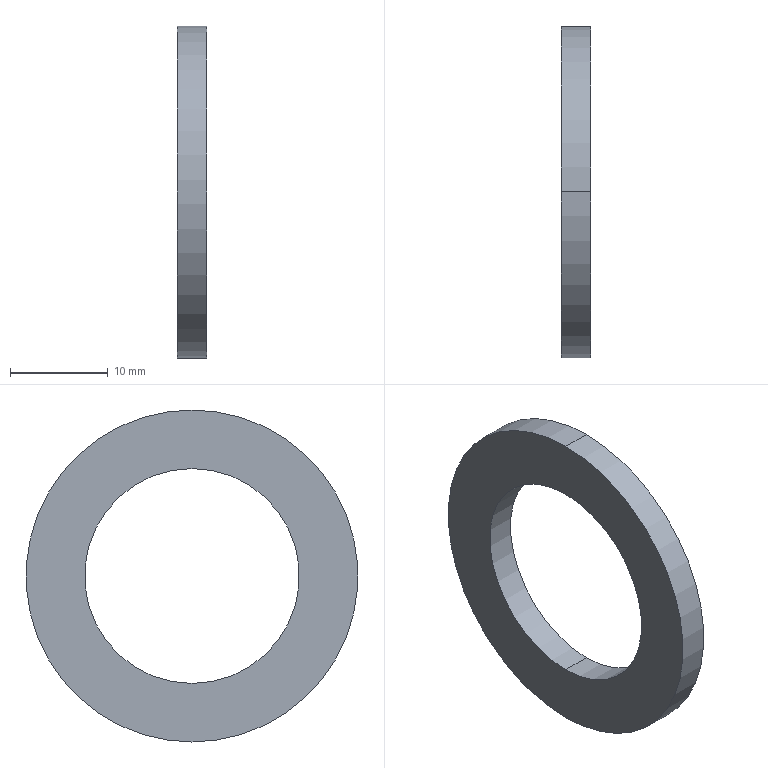Part | STEP file | Completa.sldasm-Part-113_Valor predeterminado | 1 solid | 6 faces | box 3 x 34 x 34 mm | volume 1583 mm3 | cylinder 4 | plane 2 | commonest cylinder face diameters 22 x2 34 x2
STEP:
#1=CARTESIAN_POINT('',(0.,0.,0.));
#2=DIRECTION('',(0.,0.,1.));
#3=DIRECTION('',(1.,0.,0.));
#4=AXIS2_PLACEMENT_3D('',#1,#2,#3);
#5=CARTESIAN_POINT('',(-203.167,0.,17.));
#6=VERTEX_POINT('',#5);
#7=CARTESIAN_POINT('',(-203.167,0.,-17.));
#8=VERTEX_POINT('',#7);
#9=CARTESIAN_POINT('',(-203.167,0.,0.));
#10=DIRECTION('',(-1.,0.,0.));
#11=DIRECTION('',(0.,0.,1.));
#12=AXIS2_PLACEMENT_3D('',#9,#10,#11);
#13=CIRCLE('',#12,17.);
#14=CARTESIAN_POINT('',(-203.167,0.,0.));
#15=DIRECTION('',(-1.,0.,0.));
#16=DIRECTION('',(0.,0.,1.));
#17=AXIS2_PLACEMENT_3D('',#14,#15,#16);
#18=CYLINDRICAL_SURFACE('',#17,17.);
#19=CARTESIAN_POINT('',(0.,0.));
#20=DIRECTION('',(1.,0.));
#21=VECTOR('',#20,1.);
#22=LINE('',#19,#21);
#23=(GEOMETRIC_REPRESENTATION_CONTEXT(2)PARAMETRIC_REPRESENTATION_CONTEXT()REPRESENTATION_CONTEXT('',''));
#24=DEFINITIONAL_REPRESENTATION('',(#22),#23);
#25=PCURVE('',#18,#24);
#26=CARTESIAN_POINT('',(-203.167,0.,0.));
#27=DIRECTION('',(1.,0.,0.));
#28=DIRECTION('',(0.,0.,-1.));
#29=AXIS2_PLACEMENT_3D('',#26,#27,#28);
#30=PLANE('',#29);
#31=CARTESIAN_POINT('',(-17.,0.));
#32=CARTESIAN_POINT('',(-17.,29.445));
#33=CARTESIAN_POINT('',(8.5,14.722));
#34=CARTESIAN_POINT('',(34.,0.));
#35=CARTESIAN_POINT('',(8.5,-14.722));
#36=CARTESIAN_POINT('',(-17.,-29.445));
#37=CARTESIAN_POINT('',(-17.,0.));
#38=(BOUNDED_CURVE()B_SPLINE_CURVE(2,(#31,#32,#33,#34,#35,#36,#37),.UNSPECIFIED.,.T.,.F.)B_SPLINE_CURVE_WITH_KNOTS((1,2,2,2,2,1),(-2.094,0.,2.094,4.189,6.283,8.378),.UNSPECIFIED.)CURVE()GEOMETRIC_REPRESENTATION_ITEM()RATIONAL_B_SPLINE_CURVE((1.,0.5,1.,0.5,1.,0.5,1.))REPRESENTATION_ITEM(''));
#39=(GEOMETRIC_REPRESENTATION_CONTEXT(2)PARAMETRIC_REPRESENTATION_CONTEXT()REPRESENTATION_CONTEXT('',''));
#40=DEFINITIONAL_REPRESENTATION('',(#38),#39);
#41=PCURVE('',#30,#40);
#42=SURFACE_CURVE('',#13,(#25,#41),.PCURVE_S1.);
#43=EDGE_CURVE('',#6,#8,#42,.T.);
#44=ORIENTED_EDGE('',*,*,#43,.T.);
#45=CARTESIAN_POINT('',(-206.167,0.,-17.));
#46=VERTEX_POINT('',#45);
#47=CARTESIAN_POINT('',(-203.167,0.,-17.));
#48=DIRECTION('',(-1.,0.,0.));
#49=VECTOR('',#48,1.);
#50=LINE('',#47,#49);
#51=CARTESIAN_POINT('',(3.142,0.));
#52=DIRECTION('',(0.,1.));
#53=VECTOR('',#52,1.);
#54=LINE('',#51,#53);
#55=(GEOMETRIC_REPRESENTATION_CONTEXT(2)PARAMETRIC_REPRESENTATION_CONTEXT()REPRESENTATION_CONTEXT('',''));
#56=DEFINITIONAL_REPRESENTATION('',(#54),#55);
#57=PCURVE('',#18,#56);
#58=CARTESIAN_POINT('',(-203.167,0.,0.));
#59=DIRECTION('',(-1.,0.,0.));
#60=DIRECTION('',(0.,0.,1.));
#61=AXIS2_PLACEMENT_3D('',#58,#59,#60);
#62=CYLINDRICAL_SURFACE('',#61,17.);
#63=CARTESIAN_POINT('',(3.142,0.));
#64=DIRECTION('',(0.,1.));
#65=VECTOR('',#64,1.);
#66=LINE('',#63,#65);
#67=(GEOMETRIC_REPRESENTATION_CONTEXT(2)PARAMETRIC_REPRESENTATION_CONTEXT()REPRESENTATION_CONTEXT('',''));
#68=DEFINITIONAL_REPRESENTATION('',(#66),#67);
#69=PCURVE('',#62,#68);
#70=SURFACE_CURVE('',#50,(#57,#69),.PCURVE_S1.);
#71=EDGE_CURVE('',#8,#46,#70,.T.);
#72=ORIENTED_EDGE('',*,*,#71,.T.);
#73=CARTESIAN_POINT('',(-206.167,0.,17.));
#74=VERTEX_POINT('',#73);
#75=CARTESIAN_POINT('',(-206.167,0.,0.));
#76=DIRECTION('',(-1.,0.,0.));
#77=DIRECTION('',(0.,0.,1.));
#78=AXIS2_PLACEMENT_3D('',#75,#76,#77);
#79=CIRCLE('',#78,17.);
#80=CARTESIAN_POINT('',(0.,3.));
#81=DIRECTION('',(1.,0.));
#82=VECTOR('',#81,1.);
#83=LINE('',#80,#82);
#84=(GEOMETRIC_REPRESENTATION_CONTEXT(2)PARAMETRIC_REPRESENTATION_CONTEXT()REPRESENTATION_CONTEXT('',''));
#85=DEFINITIONAL_REPRESENTATION('',(#83),#84);
#86=PCURVE('',#18,#85);
#87=CARTESIAN_POINT('',(-206.167,0.,0.));
#88=DIRECTION('',(1.,0.,0.));
#89=DIRECTION('',(0.,0.,-1.));
#90=AXIS2_PLACEMENT_3D('',#87,#88,#89);
#91=PLANE('',#90);
#92=CARTESIAN_POINT('',(-17.,0.));
#93=CARTESIAN_POINT('',(-17.,29.445));
#94=CARTESIAN_POINT('',(8.5,14.722));
#95=CARTESIAN_POINT('',(34.,0.));
#96=CARTESIAN_POINT('',(8.5,-14.722));
#97=CARTESIAN_POINT('',(-17.,-29.445));
#98=CARTESIAN_POINT('',(-17.,0.));
#99=(BOUNDED_CURVE()B_SPLINE_CURVE(2,(#92,#93,#94,#95,#96,#97,#98),.UNSPECIFIED.,.T.,.F.)B_SPLINE_CURVE_WITH_KNOTS((1,2,2,2,2,1),(-2.094,0.,2.094,4.189,6.283,8.378),.UNSPECIFIED.)CURVE()GEOMETRIC_REPRESENTATION_ITEM()RATIONAL_B_SPLINE_CURVE((1.,0.5,1.,0.5,1.,0.5,1.))REPRESENTATION_ITEM(''));
#100=(GEOMETRIC_REPRESENTATION_CONTEXT(2)PARAMETRIC_REPRESENTATION_CONTEXT()REPRESENTATION_CONTEXT('',''));
#101=DEFINITIONAL_REPRESENTATION('',(#99),#100);
#102=PCURVE('',#91,#101);
#103=SURFACE_CURVE('',#79,(#86,#102),.PCURVE_S1.);
#104=EDGE_CURVE('',#74,#46,#103,.T.);
#105=ORIENTED_EDGE('',*,*,#104,.F.);
#106=CARTESIAN_POINT('',(-203.167,0.,17.));
#107=DIRECTION('',(-1.,0.,0.));
#108=VECTOR('',#107,1.);
#109=LINE('',#106,#108);
#110=CARTESIAN_POINT('',(0.,0.));
#111=DIRECTION('',(0.,1.));
#112=VECTOR('',#111,1.);
#113=LINE('',#110,#112);
#114=(GEOMETRIC_REPRESENTATION_CONTEXT(2)PARAMETRIC_REPRESENTATION_CONTEXT()REPRESENTATION_CONTEXT('',''));
#115=DEFINITIONAL_REPRESENTATION('',(#113),#114);
#116=PCURVE('',#18,#115);
#117=CARTESIAN_POINT('',(6.283,0.));
#118=DIRECTION('',(0.,1.));
#119=VECTOR('',#118,1.);
#120=LINE('',#117,#119);
#121=(GEOMETRIC_REPRESENTATION_CONTEXT(2)PARAMETRIC_REPRESENTATION_CONTEXT()REPRESENTATION_CONTEXT('',''));
#122=DEFINITIONAL_REPRESENTATION('',(#120),#121);
#123=PCURVE('',#62,#122);
#124=SURFACE_CURVE('',#109,(#116,#123),.PCURVE_S1.);
#125=EDGE_CURVE('',#6,#74,#124,.T.);
#126=ORIENTED_EDGE('',*,*,#125,.F.);
#127=EDGE_LOOP('',(#44,#72,#105,#126));
#128=FACE_BOUND('',#127,.T.);
#129=ADVANCED_FACE('',(#128),#18,.T.);
#130=CARTESIAN_POINT('',(-203.167,0.,11.));
#131=VERTEX_POINT('',#130);
#132=CARTESIAN_POINT('',(-206.167,0.,11.));
#133=VERTEX_POINT('',#132);
#134=CARTESIAN_POINT('',(-203.167,0.,11.));
#135=DIRECTION('',(-1.,0.,0.));
#136=VECTOR('',#135,1.);
#137=LINE('',#134,#136);
#138=CARTESIAN_POINT('',(-203.167,0.,0.));
#139=DIRECTION('',(-1.,0.,0.));
#140=DIRECTION('',(0.,0.,1.));
#141=AXIS2_PLACEMENT_3D('',#138,#139,#140);
#142=CYLINDRICAL_SURFACE('',#141,11.);
#143=CARTESIAN_POINT('',(6.283,0.));
#144=DIRECTION('',(0.,1.));
#145=VECTOR('',#144,1.);
#146=LINE('',#143,#145);
#147=(GEOMETRIC_REPRESENTATION_CONTEXT(2)PARAMETRIC_REPRESENTATION_CONTEXT()REPRESENTATION_CONTEXT('',''));
#148=DEFINITIONAL_REPRESENTATION('',(#146),#147);
#149=PCURVE('',#142,#148);
#150=CARTESIAN_POINT('',(-203.167,0.,0.));
#151=DIRECTION('',(-1.,0.,0.));
#152=DIRECTION('',(0.,0.,1.));
#153=AXIS2_PLACEMENT_3D('',#150,#151,#152);
#154=CYLINDRICAL_SURFACE('',#153,11.);
#155=CARTESIAN_POINT('',(0.,0.));
#156=DIRECTION('',(0.,1.));
#157=VECTOR('',#156,1.);
#158=LINE('',#155,#157);
#159=(GEOMETRIC_REPRESENTATION_CONTEXT(2)PARAMETRIC_REPRESENTATION_CONTEXT()REPRESENTATION_CONTEXT('',''));
#160=DEFINITIONAL_REPRESENTATION('',(#158),#159);
#161=PCURVE('',#154,#160);
#162=SURFACE_CURVE('',#137,(#149,#161),.PCURVE_S1.);
#163=EDGE_CURVE('',#131,#133,#162,.T.);
#164=ORIENTED_EDGE('',*,*,#163,.T.);
#165=CARTESIAN_POINT('',(-206.167,0.,-11.));
#166=VERTEX_POINT('',#165);
#167=CARTESIAN_POINT('',(-206.167,0.,0.));
#168=DIRECTION('',(-1.,0.,0.));
#169=DIRECTION('',(0.,0.,1.));
#170=AXIS2_PLACEMENT_3D('',#167,#168,#169);
#171=CIRCLE('',#170,11.);
#172=CARTESIAN_POINT('',(0.,3.));
#173=DIRECTION('',(1.,0.));
#174=VECTOR('',#173,1.);
#175=LINE('',#172,#174);
#176=(GEOMETRIC_REPRESENTATION_CONTEXT(2)PARAMETRIC_REPRESENTATION_CONTEXT()REPRESENTATION_CONTEXT('',''));
#177=DEFINITIONAL_REPRESENTATION('',(#175),#176);
#178=PCURVE('',#142,#177);
#179=CARTESIAN_POINT('',(-11.,0.));
#180=CARTESIAN_POINT('',(-11.,19.053));
#181=CARTESIAN_POINT('',(5.5,9.526));
#182=CARTESIAN_POINT('',(22.,0.));
#183=CARTESIAN_POINT('',(5.5,-9.526));
#184=CARTESIAN_POINT('',(-11.,-19.053));
#185=CARTESIAN_POINT('',(-11.,0.));
#186=(BOUNDED_CURVE()B_SPLINE_CURVE(2,(#179,#180,#181,#182,#183,#184,#185),.UNSPECIFIED.,.T.,.F.)B_SPLINE_CURVE_WITH_KNOTS((1,2,2,2,2,1),(-2.094,0.,2.094,4.189,6.283,8.378),.UNSPECIFIED.)CURVE()GEOMETRIC_REPRESENTATION_ITEM()RATIONAL_B_SPLINE_CURVE((1.,0.5,1.,0.5,1.,0.5,1.))REPRESENTATION_ITEM(''));
#187=(GEOMETRIC_REPRESENTATION_CONTEXT(2)PARAMETRIC_REPRESENTATION_CONTEXT()REPRESENTATION_CONTEXT('',''));
#188=DEFINITIONAL_REPRESENTATION('',(#186),#187);
#189=PCURVE('',#91,#188);
#190=SURFACE_CURVE('',#171,(#178,#189),.PCURVE_S1.);
#191=EDGE_CURVE('',#166,#133,#190,.T.);
#192=ORIENTED_EDGE('',*,*,#191,.F.);
#193=CARTESIAN_POINT('',(-203.167,0.,-11.));
#194=VERTEX_POINT('',#193);
#195=CARTESIAN_POINT('',(-203.167,0.,-11.));
#196=DIRECTION('',(-1.,0.,0.));
#197=VECTOR('',#196,1.);
#198=LINE('',#195,#197);
#199=CARTESIAN_POINT('',(3.142,0.));
#200=DIRECTION('',(0.,1.));
#201=VECTOR('',#200,1.);
#202=LINE('',#199,#201);
#203=(GEOMETRIC_REPRESENTATION_CONTEXT(2)PARAMETRIC_REPRESENTATION_CONTEXT()REPRESENTATION_CONTEXT('',''));
#204=DEFINITIONAL_REPRESENTATION('',(#202),#203);
#205=PCURVE('',#142,#204);
#206=CARTESIAN_POINT('',(3.142,0.));
#207=DIRECTION('',(0.,1.));
#208=VECTOR('',#207,1.);
#209=LINE('',#206,#208);
#210=(GEOMETRIC_REPRESENTATION_CONTEXT(2)PARAMETRIC_REPRESENTATION_CONTEXT()REPRESENTATION_CONTEXT('',''));
#211=DEFINITIONAL_REPRESENTATION('',(#209),#210);
#212=PCURVE('',#154,#211);
#213=SURFACE_CURVE('',#198,(#205,#212),.PCURVE_S1.);
#214=EDGE_CURVE('',#194,#166,#213,.T.);
#215=ORIENTED_EDGE('',*,*,#214,.F.);
#216=CARTESIAN_POINT('',(-203.167,0.,0.));
#217=DIRECTION('',(-1.,0.,0.));
#218=DIRECTION('',(0.,0.,1.));
#219=AXIS2_PLACEMENT_3D('',#216,#217,#218);
#220=CIRCLE('',#219,11.);
#221=CARTESIAN_POINT('',(0.,0.));
#222=DIRECTION('',(1.,0.));
#223=VECTOR('',#222,1.);
#224=LINE('',#221,#223);
#225=(GEOMETRIC_REPRESENTATION_CONTEXT(2)PARAMETRIC_REPRESENTATION_CONTEXT()REPRESENTATION_CONTEXT('',''));
#226=DEFINITIONAL_REPRESENTATION('',(#224),#225);
#227=PCURVE('',#142,#226);
#228=CARTESIAN_POINT('',(-11.,0.));
#229=CARTESIAN_POINT('',(-11.,19.053));
#230=CARTESIAN_POINT('',(5.5,9.526));
#231=CARTESIAN_POINT('',(22.,0.));
#232=CARTESIAN_POINT('',(5.5,-9.526));
#233=CARTESIAN_POINT('',(-11.,-19.053));
#234=CARTESIAN_POINT('',(-11.,0.));
#235=(BOUNDED_CURVE()B_SPLINE_CURVE(2,(#228,#229,#230,#231,#232,#233,#234),.UNSPECIFIED.,.T.,.F.)B_SPLINE_CURVE_WITH_KNOTS((1,2,2,2,2,1),(-2.094,0.,2.094,4.189,6.283,8.378),.UNSPECIFIED.)CURVE()GEOMETRIC_REPRESENTATION_ITEM()RATIONAL_B_SPLINE_CURVE((1.,0.5,1.,0.5,1.,0.5,1.))REPRESENTATION_ITEM(''));
#236=(GEOMETRIC_REPRESENTATION_CONTEXT(2)PARAMETRIC_REPRESENTATION_CONTEXT()REPRESENTATION_CONTEXT('',''));
#237=DEFINITIONAL_REPRESENTATION('',(#235),#236);
#238=PCURVE('',#30,#237);
#239=SURFACE_CURVE('',#220,(#227,#238),.PCURVE_S1.);
#240=EDGE_CURVE('',#194,#131,#239,.T.);
#241=ORIENTED_EDGE('',*,*,#240,.T.);
#242=EDGE_LOOP('',(#164,#192,#215,#241));
#243=FACE_BOUND('',#242,.F.);
#244=ADVANCED_FACE('',(#243),#142,.F.);
#245=CARTESIAN_POINT('',(-203.167,0.,0.));
#246=DIRECTION('',(-1.,0.,0.));
#247=DIRECTION('',(0.,0.,1.));
#248=AXIS2_PLACEMENT_3D('',#245,#246,#247);
#249=CIRCLE('',#248,11.);
#250=CARTESIAN_POINT('',(-11.,0.));
#251=CARTESIAN_POINT('',(-11.,19.053));
#252=CARTESIAN_POINT('',(5.5,9.526));
#253=CARTESIAN_POINT('',(22.,0.));
#254=CARTESIAN_POINT('',(5.5,-9.526));
#255=CARTESIAN_POINT('',(-11.,-19.053));
#256=CARTESIAN_POINT('',(-11.,0.));
#257=(BOUNDED_CURVE()B_SPLINE_CURVE(2,(#250,#251,#252,#253,#254,#255,#256),.UNSPECIFIED.,.T.,.F.)B_SPLINE_CURVE_WITH_KNOTS((1,2,2,2,2,1),(-2.094,0.,2.094,4.189,6.283,8.378),.UNSPECIFIED.)CURVE()GEOMETRIC_REPRESENTATION_ITEM()RATIONAL_B_SPLINE_CURVE((1.,0.5,1.,0.5,1.,0.5,1.))REPRESENTATION_ITEM(''));
#258=(GEOMETRIC_REPRESENTATION_CONTEXT(2)PARAMETRIC_REPRESENTATION_CONTEXT()REPRESENTATION_CONTEXT('',''));
#259=DEFINITIONAL_REPRESENTATION('',(#257),#258);
#260=PCURVE('',#30,#259);
#261=CARTESIAN_POINT('',(0.,0.));
#262=DIRECTION('',(1.,0.));
#263=VECTOR('',#262,1.);
#264=LINE('',#261,#263);
#265=(GEOMETRIC_REPRESENTATION_CONTEXT(2)PARAMETRIC_REPRESENTATION_CONTEXT()REPRESENTATION_CONTEXT('',''));
#266=DEFINITIONAL_REPRESENTATION('',(#264),#265);
#267=PCURVE('',#154,#266);
#268=SURFACE_CURVE('',#249,(#260,#267),.PCURVE_S1.);
#269=EDGE_CURVE('',#131,#194,#268,.T.);
#270=ORIENTED_EDGE('',*,*,#269,.T.);
#271=ORIENTED_EDGE('',*,*,#240,.T.);
#272=EDGE_LOOP('',(#270,#271));
#273=FACE_BOUND('',#272,.T.);
#274=ORIENTED_EDGE('',*,*,#43,.F.);
#275=CARTESIAN_POINT('',(-203.167,0.,0.));
#276=DIRECTION('',(-1.,0.,0.));
#277=DIRECTION('',(0.,0.,1.));
#278=AXIS2_PLACEMENT_3D('',#275,#276,#277);
#279=CIRCLE('',#278,17.);
#280=CARTESIAN_POINT('',(-17.,0.));
#281=CARTESIAN_POINT('',(-17.,29.445));
#282=CARTESIAN_POINT('',(8.5,14.722));
#283=CARTESIAN_POINT('',(34.,0.));
#284=CARTESIAN_POINT('',(8.5,-14.722));
#285=CARTESIAN_POINT('',(-17.,-29.445));
#286=CARTESIAN_POINT('',(-17.,0.));
#287=(BOUNDED_CURVE()B_SPLINE_CURVE(2,(#280,#281,#282,#283,#284,#285,#286),.UNSPECIFIED.,.T.,.F.)B_SPLINE_CURVE_WITH_KNOTS((1,2,2,2,2,1),(-2.094,0.,2.094,4.189,6.283,8.378),.UNSPECIFIED.)CURVE()GEOMETRIC_REPRESENTATION_ITEM()RATIONAL_B_SPLINE_CURVE((1.,0.5,1.,0.5,1.,0.5,1.))REPRESENTATION_ITEM(''));
#288=(GEOMETRIC_REPRESENTATION_CONTEXT(2)PARAMETRIC_REPRESENTATION_CONTEXT()REPRESENTATION_CONTEXT('',''));
#289=DEFINITIONAL_REPRESENTATION('',(#287),#288);
#290=PCURVE('',#30,#289);
#291=CARTESIAN_POINT('',(0.,0.));
#292=DIRECTION('',(1.,0.));
#293=VECTOR('',#292,1.);
#294=LINE('',#291,#293);
#295=(GEOMETRIC_REPRESENTATION_CONTEXT(2)PARAMETRIC_REPRESENTATION_CONTEXT()REPRESENTATION_CONTEXT('',''));
#296=DEFINITIONAL_REPRESENTATION('',(#294),#295);
#297=PCURVE('',#62,#296);
#298=SURFACE_CURVE('',#279,(#290,#297),.PCURVE_S1.);
#299=EDGE_CURVE('',#8,#6,#298,.T.);
#300=ORIENTED_EDGE('',*,*,#299,.F.);
#301=EDGE_LOOP('',(#274,#300));
#302=FACE_BOUND('',#301,.T.);
#303=ADVANCED_FACE('',(#273,#302),#30,.T.);
#304=CARTESIAN_POINT('',(-206.167,0.,0.));
#305=DIRECTION('',(-1.,0.,0.));
#306=DIRECTION('',(0.,0.,1.));
#307=AXIS2_PLACEMENT_3D('',#304,#305,#306);
#308=CIRCLE('',#307,11.);
#309=CARTESIAN_POINT('',(-11.,0.));
#310=CARTESIAN_POINT('',(-11.,19.053));
#311=CARTESIAN_POINT('',(5.5,9.526));
#312=CARTESIAN_POINT('',(22.,0.));
#313=CARTESIAN_POINT('',(5.5,-9.526));
#314=CARTESIAN_POINT('',(-11.,-19.053));
#315=CARTESIAN_POINT('',(-11.,0.));
#316=(BOUNDED_CURVE()B_SPLINE_CURVE(2,(#309,#310,#311,#312,#313,#314,#315),.UNSPECIFIED.,.T.,.F.)B_SPLINE_CURVE_WITH_KNOTS((1,2,2,2,2,1),(-2.094,0.,2.094,4.189,6.283,8.378),.UNSPECIFIED.)CURVE()GEOMETRIC_REPRESENTATION_ITEM()RATIONAL_B_SPLINE_CURVE((1.,0.5,1.,0.5,1.,0.5,1.))REPRESENTATION_ITEM(''));
#317=(GEOMETRIC_REPRESENTATION_CONTEXT(2)PARAMETRIC_REPRESENTATION_CONTEXT()REPRESENTATION_CONTEXT('',''));
#318=DEFINITIONAL_REPRESENTATION('',(#316),#317);
#319=PCURVE('',#91,#318);
#320=CARTESIAN_POINT('',(0.,3.));
#321=DIRECTION('',(1.,0.));
#322=VECTOR('',#321,1.);
#323=LINE('',#320,#322);
#324=(GEOMETRIC_REPRESENTATION_CONTEXT(2)PARAMETRIC_REPRESENTATION_CONTEXT()REPRESENTATION_CONTEXT('',''));
#325=DEFINITIONAL_REPRESENTATION('',(#323),#324);
#326=PCURVE('',#154,#325);
#327=SURFACE_CURVE('',#308,(#319,#326),.PCURVE_S1.);
#328=EDGE_CURVE('',#133,#166,#327,.T.);
#329=ORIENTED_EDGE('',*,*,#328,.F.);
#330=ORIENTED_EDGE('',*,*,#191,.F.);
#331=EDGE_LOOP('',(#329,#330));
#332=FACE_BOUND('',#331,.T.);
#333=ORIENTED_EDGE('',*,*,#104,.T.);
#334=CARTESIAN_POINT('',(-206.167,0.,0.));
#335=DIRECTION('',(-1.,0.,0.));
#336=DIRECTION('',(0.,0.,1.));
#337=AXIS2_PLACEMENT_3D('',#334,#335,#336);
#338=CIRCLE('',#337,17.);
#339=CARTESIAN_POINT('',(-17.,0.));
#340=CARTESIAN_POINT('',(-17.,29.445));
#341=CARTESIAN_POINT('',(8.5,14.722));
#342=CARTESIAN_POINT('',(34.,0.));
#343=CARTESIAN_POINT('',(8.5,-14.722));
#344=CARTESIAN_POINT('',(-17.,-29.445));
#345=CARTESIAN_POINT('',(-17.,0.));
#346=(BOUNDED_CURVE()B_SPLINE_CURVE(2,(#339,#340,#341,#342,#343,#344,#345),.UNSPECIFIED.,.T.,.F.)B_SPLINE_CURVE_WITH_KNOTS((1,2,2,2,2,1),(-2.094,0.,2.094,4.189,6.283,8.378),.UNSPECIFIED.)CURVE()GEOMETRIC_REPRESENTATION_ITEM()RATIONAL_B_SPLINE_CURVE((1.,0.5,1.,0.5,1.,0.5,1.))REPRESENTATION_ITEM(''));
#347=(GEOMETRIC_REPRESENTATION_CONTEXT(2)PARAMETRIC_REPRESENTATION_CONTEXT()REPRESENTATION_CONTEXT('',''));
#348=DEFINITIONAL_REPRESENTATION('',(#346),#347);
#349=PCURVE('',#91,#348);
#350=CARTESIAN_POINT('',(0.,3.));
#351=DIRECTION('',(1.,0.));
#352=VECTOR('',#351,1.);
#353=LINE('',#350,#352);
#354=(GEOMETRIC_REPRESENTATION_CONTEXT(2)PARAMETRIC_REPRESENTATION_CONTEXT()REPRESENTATION_CONTEXT('',''));
#355=DEFINITIONAL_REPRESENTATION('',(#353),#354);
#356=PCURVE('',#62,#355);
#357=SURFACE_CURVE('',#338,(#349,#356),.PCURVE_S1.);
#358=EDGE_CURVE('',#46,#74,#357,.T.);
#359=ORIENTED_EDGE('',*,*,#358,.T.);
#360=EDGE_LOOP('',(#333,#359));
#361=FACE_BOUND('',#360,.T.);
#362=ADVANCED_FACE('',(#332,#361),#91,.F.);
#363=ORIENTED_EDGE('',*,*,#328,.F.);
#364=ORIENTED_EDGE('',*,*,#163,.F.);
#365=ORIENTED_EDGE('',*,*,#269,.T.);
#366=ORIENTED_EDGE('',*,*,#214,.T.);
#367=EDGE_LOOP('',(#363,#364,#365,#366));
#368=FACE_BOUND('',#367,.F.);
#369=ADVANCED_FACE('',(#368),#154,.F.);
#370=ORIENTED_EDGE('',*,*,#71,.F.);
#371=ORIENTED_EDGE('',*,*,#299,.T.);
#372=ORIENTED_EDGE('',*,*,#125,.T.);
#373=ORIENTED_EDGE('',*,*,#358,.F.);
#374=EDGE_LOOP('',(#370,#371,#372,#373));
#375=FACE_BOUND('',#374,.T.);
#376=ADVANCED_FACE('',(#375),#62,.T.);
#377=CLOSED_SHELL('',(#129,#244,#303,#362,#369,#376));
#378=MANIFOLD_SOLID_BREP('',#377);
#379=(LENGTH_UNIT()NAMED_UNIT(*)SI_UNIT(.MILLI.,.METRE.));
#380=UNCERTAINTY_MEASURE_WITH_UNIT(LENGTH_MEASURE(0.0000001),#379,'','');
#381=(NAMED_UNIT(*)PLANE_ANGLE_UNIT()SI_UNIT($,.RADIAN.));
#382=(NAMED_UNIT(*)SI_UNIT($,.STERADIAN.)SOLID_ANGLE_UNIT());
#383=(GEOMETRIC_REPRESENTATION_CONTEXT(3)GLOBAL_UNCERTAINTY_ASSIGNED_CONTEXT((#380))GLOBAL_UNIT_ASSIGNED_CONTEXT((#379,#381,#382))REPRESENTATION_CONTEXT('',''));
#384=ADVANCED_BREP_SHAPE_REPRESENTATION('',(#4,#378),#383);